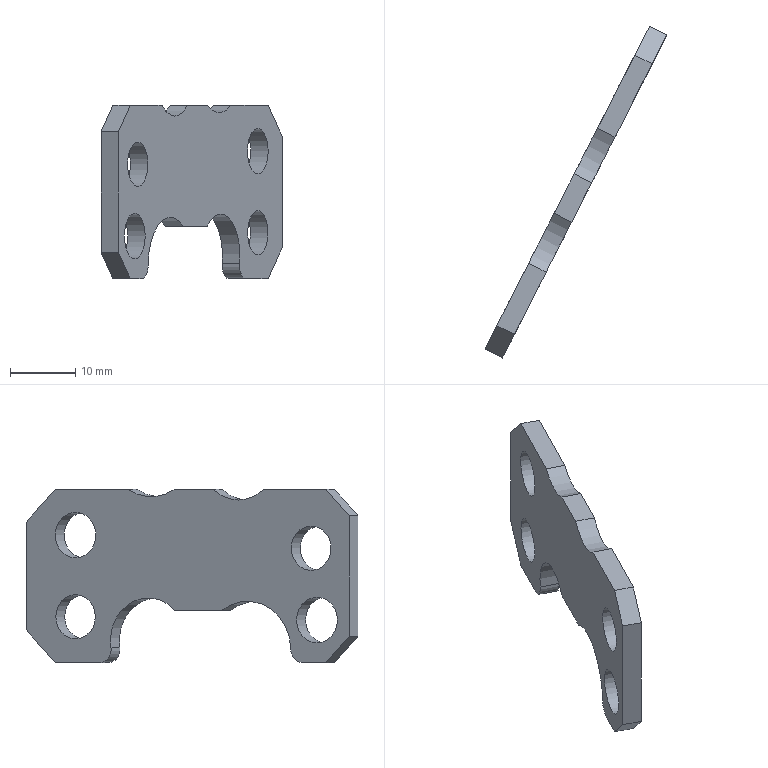Part | STEP file | gslz 2016.10.28-13_id98_x_t | 1 solid | 24 faces | box 27.869 x 50.813 x 26.5 mm | volume 3011 mm3 | plane 14 | cylinder 10 | commonest cylinder face diameters 4 x2 6.8 x2 7 x2 13 x2 15 x2